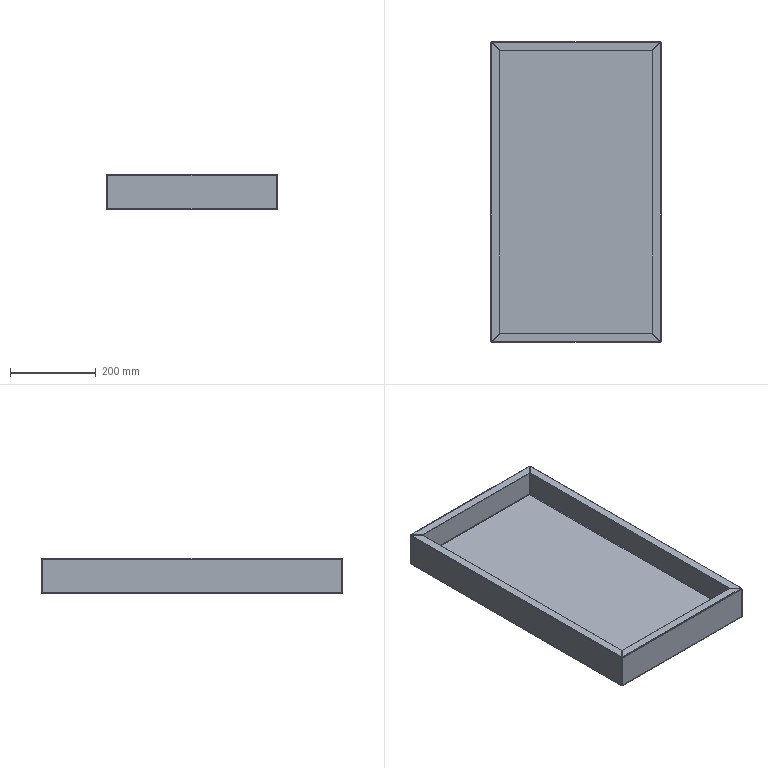Part | SolidWorks | features BaseBody 1 | 1 solid | 70 faces | box 397.4 x 702.4 x 82.4 mm | volume 594680 mm3 | plane 38 | cylinder 16 | spline 16 | commonest cylinder face diameters 2 x8 4.4 x8